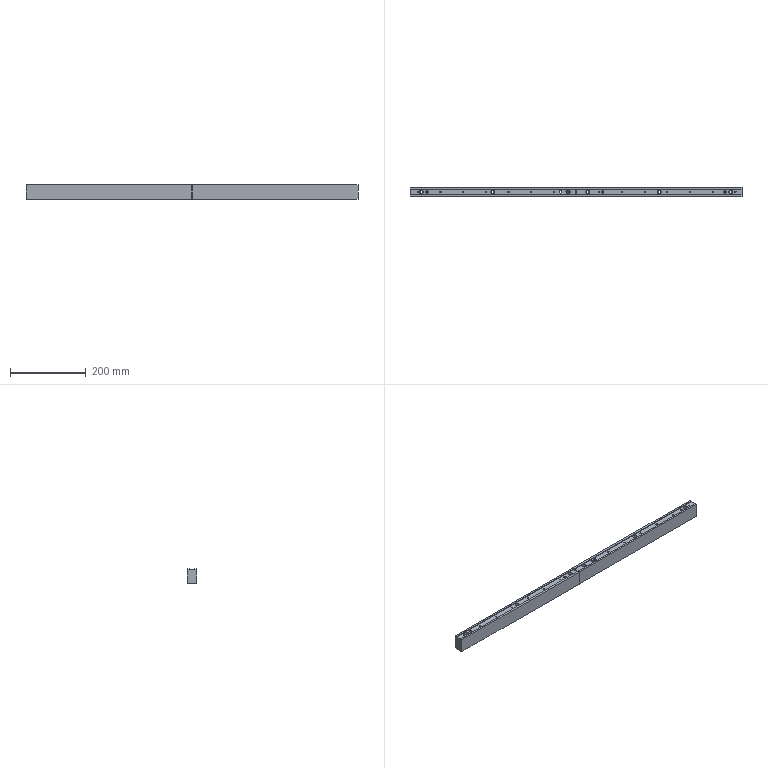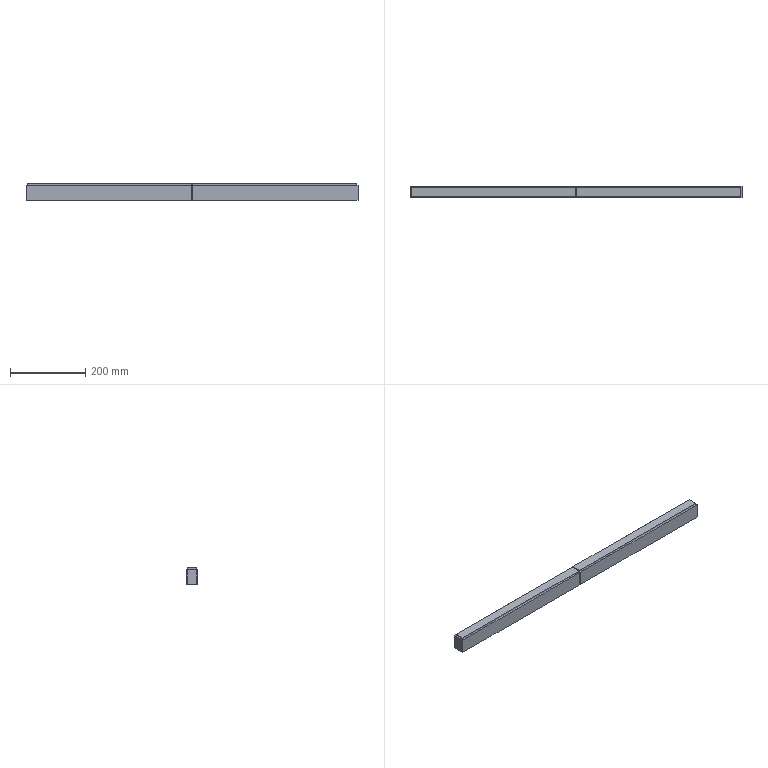CAM job | NX | 3-axis milling, drilling | part box 878 x 25 x 39 mm | stock box 884 x 31 x 44 mm
Tools:
number,name,description,diameter,corner_radius,flute_length,length,flutes
1,D63,Milling Tool-5 Parameters,63.0,0.0,50.0,75.0,2
16,6.6ZT,Drilling Tool,6.6,0.0,35.0,50.0,2
10,D10,Milling Tool-5 Parameters,10.0,0.0,50.0,75.0,2
14,5.8ZT,Drilling Tool,4.8,0.0,35.0,50.0,2
15,6.0JD,Milling Tool-5 Parameters,5.0,0.0,30.0,30.0,4
11,D10JING,Milling Tool-5 Parameters,10.0,0.0,50.0,75.0,2
7,D6A45,Milling Tool-5 Parameters,6.0,0.0,3.0,3.0,2
4,D4,Milling Tool-5 Parameters,4.0,0.0,50.0,75.0,2
13,3.3ZT,Drilling Tool,3.3,0.0,35.0,50.0,2
12,M4,Milling Tool-5 Parameters,3.3,0.0,30.0,30.0,4
6,D6,Milling Tool-5 Parameters,6.0,0.0,50.0,75.0,2
Operations:
program,operation,operation_type,tool,method,geometry_group,spindle_rpm,surface_speed,feed_per_tooth,feed_cut,feed_plunge,cut_length_mm,path_length_mm,cut_time_min,machine_time_min
1-441-45-30毛胚,FLOOR_WALL,VolumeBased25DMillingOperation,D63,METHOD,A,6500.0,1286.0,0.0962,1250.0,100.0,519.0,573.0,0.4152,0.4206
1-441-45-30毛胚,DRILLING_COPY_1,Operation,D6A45,METHOD,A,3000.0,56.0,0.0333,200.0,0.0,20.0,500.577,0.1,0.1481
1-441-45-30毛胚,DRILLING_COPY_1_COPY_COPY_COPY_COPY,Operation,6.6ZT,METHOD,A,2000.0,20.0,0.0375,150.0,0.0,131.948,717.943,0.8797,0.9383
1-441-45-30毛胚,DRILLING_COPY_1_COPY_COPY,Operation,5.8ZT,METHOD,A,2000.0,15.0,0.0375,150.0,0.0,85.884,588.281,0.5726,0.6228
1-441-45-30毛胚,DRILLING_COPY_1_COPY_COPY_COPY_COPY_1,Operation,6.0JD,METHOD,A,1000.0,15.0,0.0125,50.0,0.0,40.5,141.0,0.81,0.8201
1-441-45-30毛胚,ADAPTIVE_MILLING,CavityMilling,D10,METHOD,A,7000.0,219.0,0.2143,3000.0,1000.0,5807.189,6041.729,1.94,1.963
1-441-45-30毛胚,ZLEVEL_PROFILE_COPY_COPY_1,ZLevelMilling,D10JING,METHOD,A,7000.0,219.0,0.0714,1000.0,100.0,1938.617,2077.72,1.939,1.952
1-441-45-30毛胚,ZLEVEL_PROFILE,ZLevelMilling,D4,METHOD,A,7000.0,87.0,0.0857,1200.0,1000.0,1027.313,1121.313,0.8618,0.8712
1-441-45-30毛胚,ZLEVEL_PROFILE_COPY_1_COPY_COPY_COPY_COPY_2_COPY_COPY,ZLevelMilling,D6A45,METHOD,A,7000.0,131.0,0.0714,1000.0,1000.0,1022.923,2190.767,1.023,1.14
1-441-45-30毛胚,刀补11,ZLevelMilling,D4,METHOD,A,7000.0,219.0,0.0714,1000.0,100.0,85.035,218.451,0.085,0.0984
2-441-45-30毛胚,FLOOR_WALL_COPY,VolumeBased25DMillingOperation,D63,METHOD,B,6500.0,1286.0,0.0962,1250.0,100.0,2565.0,4843.001,2.052,2.28
2-441-45-30毛胚,ZLEVEL_PROFILE_COPY_COPY_1_COPY,ZLevelMilling,D10,METHOD,B,7000.0,219.0,0.1429,2000.0,100.0,1853.966,2444.497,0.927,0.986
2-441-45-30毛胚,DRILLING_COPY_1_COPY,Operation,D6A45,METHOD,B,3000.0,56.0,0.0333,200.0,0.0,35.7,513.85,0.1785,0.2263
2-441-45-30毛胚,DRILLING_COPY_1_COPY_COPY_COPY,Operation,3.3ZT,METHOD,B,1000.0,15.0,0.0125,50.0,0.0,98.64,639.73,1.973,2.027
2-441-45-30毛胚,DRILLING_COPY_1_COPY_COPY_COPY_COPY_1_1,Operation,M4,METHOD,B,200.0,2.0,0.0009,0.7,0.0,91.7,625.85,131.0,131.053
2-441-45-30毛胚,HOLE_MILLING,CylinderMilling,D6,METHOD,B,7000.0,131.0,0.1071,1500.0,100.0,721.325,1319.025,0.4809,0.5407
2-441-45-30毛胚,ZLEVEL_PROFILE_COPY_1_COPY_COPY_COPY_COPY_2_COPY_COPY_COPY,ZLevelMilling,D6A45,METHOD,B,7000.0,131.0,0.0714,1000.0,1000.0,1790.2,2353.065,1.79,1.847
2-441-45-30毛胚,ZLEVEL_PROFILE_COPY_1_COPY_COPY_COPY_COPY_2_COPY_COPY_COPY_COPY,ZLevelMilling,D6A45,METHOD,B,7000.0,131.0,0.0714,1000.0,1000.0,186.59,3722.856,0.1866,0.5402
2-441-45-30毛胚,刀补11_1,ZLevelMilling,D10JING,METHOD,B,7000.0,219.0,0.0714,1000.0,100.0,931.144,1055.24,0.9311,0.9436
11-441-45-30毛胚,FLOOR_WALL_COPY_1,VolumeBased25DMillingOperation,D63,METHOD,AA,6500.0,1286.0,0.0962,1250.0,100.0,519.0,573.0,0.4152,0.4206
11-441-45-30毛胚,DRILLING_COPY_1_COPY_1,Operation,D6A45,METHOD,AA,3000.0,56.0,0.0333,200.0,0.0,20.0,490.456,0.1,0.147
11-441-45-30毛胚,DRILLING_COPY_1_COPY_COPY_COPY_COPY_COPY,Operation,6.6ZT,METHOD,AA,2000.0,20.0,0.0375,150.0,0.0,131.948,707.945,0.8797,0.9373
11-441-45-30毛胚,DRILLING_COPY_1_COPY_COPY_COPY_1,Operation,5.8ZT,METHOD,AA,2000.0,15.0,0.0375,150.0,0.0,85.884,557.282,0.5726,0.6197
11-441-45-30毛胚,DRILLING_COPY_1_COPY_COPY_COPY_COPY_1_COPY,Operation,6.0JD,METHOD,AA,1000.0,15.0,0.0125,50.0,0.0,40.5,141.0,0.81,0.8201
11-441-45-30毛胚,ADAPTIVE_MILLING_COPY,CavityMilling,D10,METHOD,AA,7000.0,219.0,0.2143,3000.0,1000.0,5807.189,6041.729,1.94,1.963
11-441-45-30毛胚,ZLEVEL_PROFILE_COPY_COPY_1_COPY_1,ZLevelMilling,D10JING,METHOD,AA,7000.0,219.0,0.0714,1000.0,100.0,1938.617,2077.72,1.939,1.952
11-441-45-30毛胚,ZLEVEL_PROFILE_COPY,ZLevelMilling,D4,METHOD,AA,7000.0,87.0,0.0857,1200.0,1000.0,1027.313,1121.313,0.8618,0.8712
11-441-45-30毛胚,ZLEVEL_PROFILE_COPY_1_COPY_COPY_COPY_COPY_2_COPY_COPY_COPY_1,ZLevelMilling,D6A45,METHOD,AA,7000.0,131.0,0.0714,1000.0,1000.0,1022.923,2521.876,1.023,1.173
11-441-45-30毛胚,刀补11_COPY,ZLevelMilling,D4,METHOD,AA,7000.0,219.0,0.0714,1000.0,100.0,85.035,218.451,0.085,0.0984
22-441-45-30毛胚,FLOOR_WALL_COPY_COPY,VolumeBased25DMillingOperation,D63,METHOD,BB,6500.0,1286.0,0.0962,1250.0,100.0,2565.0,4843.001,2.052,2.28
22-441-45-30毛胚,ZLEVEL_PROFILE_COPY_COPY_1_COPY_COPY,ZLevelMilling,D10,METHOD,BB,7000.0,219.0,0.1429,2000.0,100.0,1853.831,2444.353,0.9269,0.986
22-441-45-30毛胚,DRILLING_COPY_1_COPY_COPY_1,Operation,D6A45,METHOD,BB,3000.0,56.0,0.0333,200.0,0.0,35.7,513.85,0.1785,0.2263
22-441-45-30毛胚,DRILLING_COPY_1_COPY_COPY_COPY_COPY_2,Operation,3.3ZT,METHOD,BB,1000.0,15.0,0.0125,50.0,0.0,98.64,639.73,1.973,2.027
22-441-45-30毛胚,DRILLING_COPY_1_COPY_COPY_COPY_COPY_1_1_COPY,Operation,M4,METHOD,BB,200.0,2.0,0.0009,0.7,0.0,91.7,625.85,131.0,131.053
22-441-45-30毛胚,HOLE_MILLING_COPY,CylinderMilling,D6,METHOD,BB,7000.0,131.0,0.1071,1500.0,100.0,721.325,1309.025,0.4809,0.5397
22-441-45-30毛胚,ZLEVEL_PROFILE_COPY_1_COPY_COPY_COPY_COPY_2_COPY_COPY_COPY_COPY_1,ZLevelMilling,D6A45,METHOD,BB,7000.0,131.0,0.0714,1000.0,1000.0,1790.2,2353.065,1.79,1.847
22-441-45-30毛胚,ZLEVEL_PROFILE_COPY_1_COPY_COPY_COPY_COPY_2_COPY_COPY_COPY_COPY_COPY,ZLevelMilling,D6A45,METHOD,BB,7000.0,131.0,0.0714,1000.0,1000.0,186.571,3702.487,0.1866,0.5382
22-441-45-30毛胚,刀补11_1_COPY,ZLevelMilling,D10JING,METHOD,BB,7000.0,219.0,0.0714,1000.0,100.0,931.118,1055.212,0.9311,0.9435